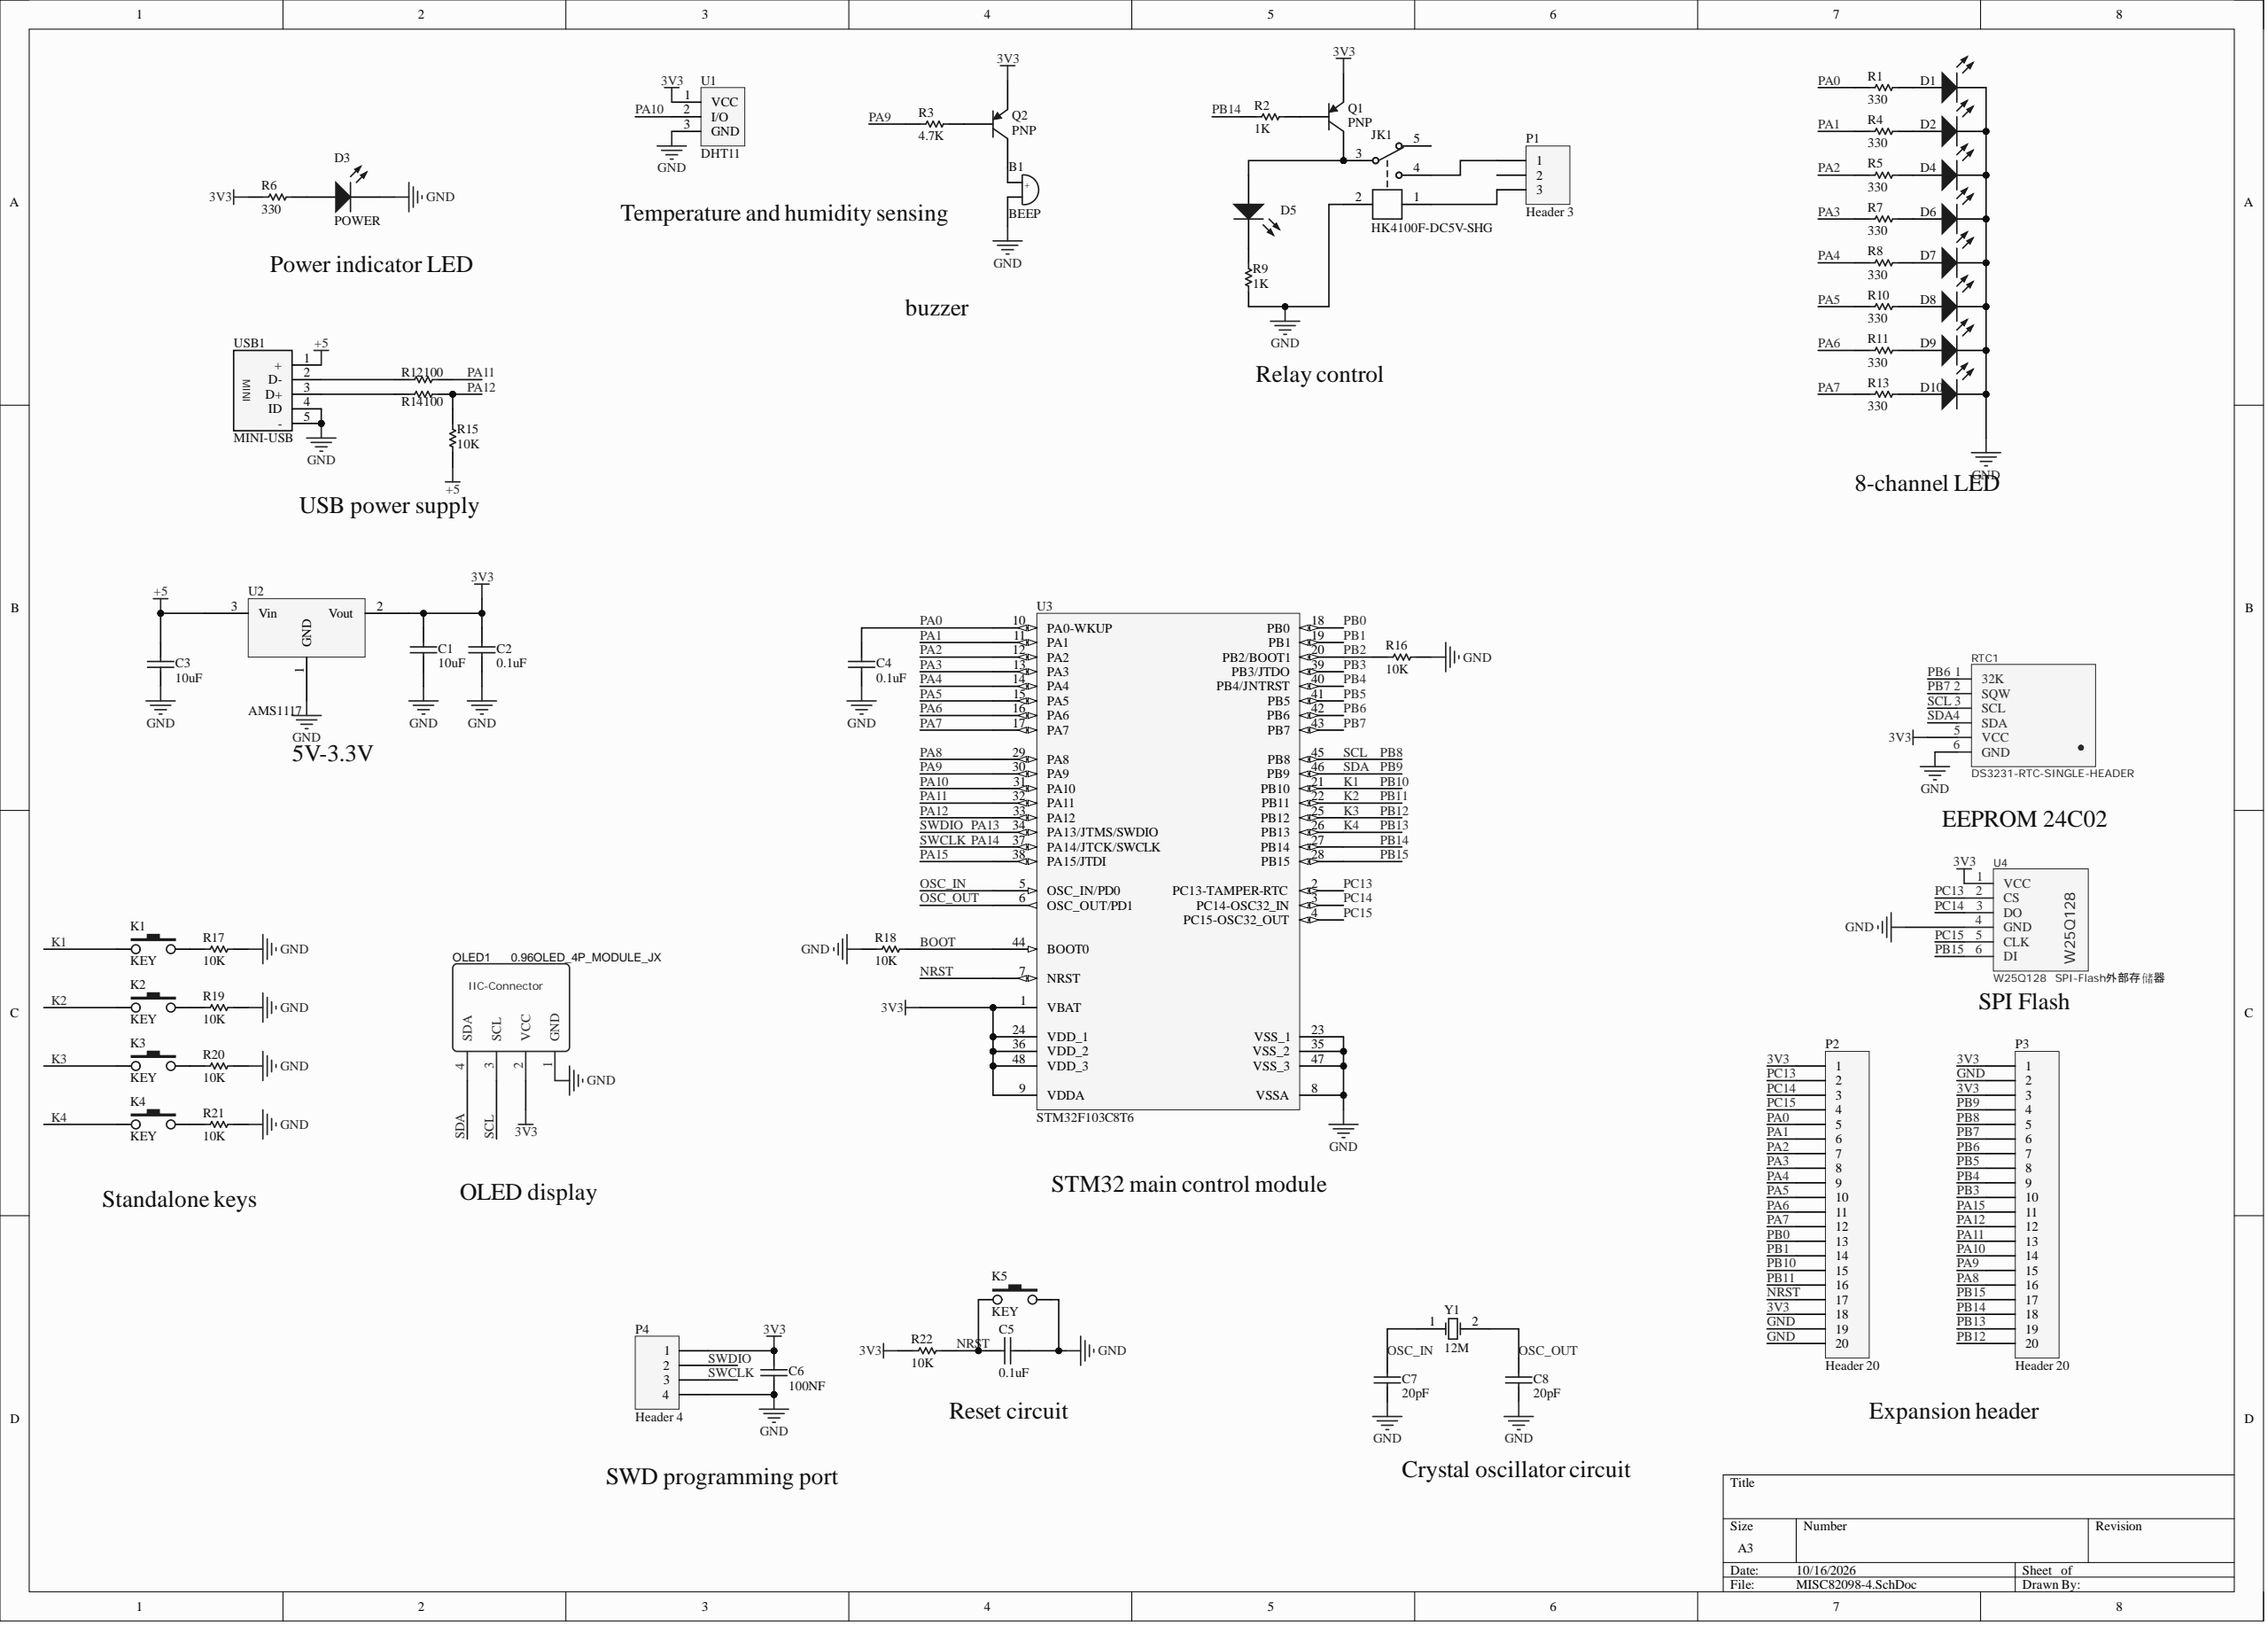Circuit board | Altium Designer | 61 parts | 64 nets
Bill of materials:
Comment,Description,Designator,Footprint,LibRef,Quantity
"BEEP","buzzer","B1","HDR1X2","BEEP","1"
"10uF","non-polarized capacitor","C1, C3","C0603","CAP","2"
"0.1uF","non-polarized capacitor","C2, C4, C5","C0603","CAP","3"
"100NF","non-polarized capacitor","C6","C0603","CAP","1"
"20pF","non-polarized capacitor","C7, C8","C0603","CAP","2"
"POWER","Typical RED, GREEN, YELLOW, AMBER GaAs LED","D1, D2, D3, D4, D5, D6, D7, D8, D9, D10","3.2X1.6X1.1","LED2","10"
"HK4100F-DC5V-SHG","changeover switch set","JK1","HK4100F","HK4100F","1"
"KEY","","K1, K2, K3, K4, K5","DIP-3X6X4.3","KEY","5"
"0.96OLED_4P_MODULE_JX","","OLED1","0.96OLED_4P","0.96OLED_4P_MODULE_JX","1"
"Header 3","Header, 3-Pin","P1","HDR1X3","Header 3","1"
"Header 20","Header, 20-Pin","P2, P3","HDR1X20","Header 20","2"
"Header 4","Header, 4-Pin","P4","HDR1X4","Header 4","1"
"PNP","PNP Bipolar Transistor","Q1, Q2","SOT-23B_N","PNP","2"
"330","","R1, R4, R5, R6, R7, R8, R10, R11, R13","6-0805_N","RES","9"
"1K","","R2, R9","6-0805_N","RES","2"
"4.7K","","R3","6-0805_N","RES","1"
"100","","R12, R14","6-0805_N","RES","2"
"10K","","R15, R16, R17, R18, R19, R20, R21, R22","6-0805_N","RES","8"
"DS3231-RTC-SINGLE-HEADER","","RTC1","DS3231-RTC-24C32-EEPROM-SINGLE-HEADER","DS3231-RTC-SINGLE-HEADER","1"
"DHT11","Header, 3-Pin","U1","HDR1X3","Header 3","1"
"AMS1117","three-terminal voltage regulator","U2","SOT223","AMS1117","1"
"STM32F103C8T6","","U3","LQFP48 7X7","STM32F103C8T6","1"
"W25Q128  SPI-Flash外部存储器","","U4","SPI FLASH","W25Q128  SPI-Flash外部存储器","1"
"MINI-USB","","USB1","USB-MINI-A","MINI-USB","1"
"12M","Crystal Oscillator","Y1","XTAL_US","XTAL","1"
Netlist (Protel format):
[
B1
HDR1X2
BEEP



]
[
C1
C0603
10uF



]
[
C2
C0603
0.1uF



]
[
C3
C0603
10uF



]
[
C4
C0603
0.1uF



]
[
C5
C0603
0.1uF



]
[
C6
C0603
100NF



]
[
C7
C0603
20pF



]
[
C8
C0603
20pF



]
[
D1
3.2X1.6X1.1
POWER



]
[
D2
3.2X1.6X1.1
POWER



]
[
D3
3.2X1.6X1.1
POWER



]
[
D4
3.2X1.6X1.1
POWER



]
[
D5
3.2X1.6X1.1
POWER



]
[
D6
3.2X1.6X1.1
POWER



]
[
D7
3.2X1.6X1.1
POWER



]
[
D8
3.2X1.6X1.1
POWER



]
[
D9
3.2X1.6X1.1
POWER



]
[
D10
3.2X1.6X1.1
POWER



]
[
JK1
HK4100F
HK4100F-DC5V-SHG



]
[
K1
DIP-3X6X4.3
KEY



]
[
K2
DIP-3X6X4.3
KEY



]
[
K3
DIP-3X6X4.3
KEY



]
[
K4
DIP-3X6X4.3
KEY



]
[
K5
DIP-3X6X4.3
KEY



]
[
OLED1
0.96OLED_4P
0.96OLED_4P_MODULE_JX



]
[
P1
HDR1X3
Header 3



]
[
P2
HDR1X20
Header 20



]
[
P3
HDR1X20
Header 20



]
[
P4
HDR1X4
Header 4



]
[
Q1
SOT-23B_N
PNP



]
[
Q2
SOT-23B_N
PNP



]
[
R1
6-0805_N
330



]
[
R2
6-0805_N
1K



]
[
R3
6-0805_N
4.7K



]
[
R4
6-0805_N
330



]
[
R5
6-0805_N
330



]
[
R6
6-0805_N
330



]
[
R7
6-0805_N
330



]
[
R8
6-0805_N
330



]
[
R9
6-0805_N
1K



]
[
R10
6-0805_N
330



]
[
R11
6-0805_N
330



]
[
R12
6-0805_N
100



]
[
R13
6-0805_N
330



]
[
R14
6-0805_N
100



]
[
R15
6-0805_N
10K



]
[
R16
6-0805_N
10K



]
[
R17
6-0805_N
10K



]
[
R18
6-0805_N
10K



]
[
R19
6-0805_N
10K



]
[
R20
6-0805_N
10K



]
[
R21
6-0805_N
10K



]
[
R22
6-0805_N
10K



]
[
RTC1
DS3231-RTC-24C32-EEPROM-SINGLE-HEADER
DS3231-RTC-SINGLE-HEADER



]
[
U1
HDR1X3
DHT11



]
[
U2
SOT223
AMS1117



]
[
U3
LQFP48 7X7
STM32F103C8T6



]
[
U4
SPI FLASH
W25Q128  SPI-Flash外部存储器



]
[
USB1
USB-MINI-A
MINI-USB



]
[
Y1
XTAL_US
12M



]
(
PC15
P2-4
U3-4
U4-5
)
(
PC14
P2-3
U3-3
U4-3
)
(
PC13
P2-2
U3-2
U4-2
)
(
PB15
P3-17
U3-28
U4-6
)
(
PB14
P3-18
R2-2
U3-27
)
(
PB9
OLED1-4
P3-4
RTC1-4
U3-46
)
(
PB8
OLED1-3
P3-5
RTC1-3
U3-45
)
(
PB7
P3-6
RTC1-2
U3-43
)
(
PB6
P3-7
RTC1-1
U3-42
)
(
PB5
P3-8
U3-41
)
(
PB4
P3-9
U3-40
)
(
PB3
P3-10
U3-39
)
(
PB2
R16-2
U3-20
)
(
PB1
P2-14
U3-19
)
(
PB0
P2-13
U3-18
)
(
PA15
P3-11
U3-38
)
(
PA14
P4-3
U3-37
)
(
PA13
P4-2
U3-34
)
(
PA12
P3-12
R14-1
R15-1
U3-33
)
(
PA11
P3-13
R12-1
U3-32
)
(
PA10
P3-14
U1-2
U3-31
)
(
PA9
P3-15
R3-2
U3-30
)
(
PA8
P3-16
U3-29
)
(
PA7
P2-12
R13-2
U3-17
)
(
PA6
P2-11
R11-2
U3-16
)
(
PA5
P2-10
R10-2
U3-15
)
(
PA4
P2-9
R8-2
U3-14
)
(
PA3
P2-8
R7-2
U3-13
)
(
PA2
P2-7
R5-2
U3-12
)
(
PA1
P2-6
R4-2
U3-11
)
(
PA0
C4-2
P2-5
R1-2
U3-10
)
(
OSC_OUT
C8-2
U3-6
Y1-2
)
(
OSC_IN
C7-2
U3-5
Y1-1
)
(
NRST
C5-2
K5-1
P2-17
R22-1
U3-7
)
(
NetR14_2
R14-2
USB1-3
)
(
NetR12_2
R12-2
USB1-2
)
(
NetQ2_2
Q2-2
R3-1
)
(
NetQ1_2
Q1-2
R2-1
)
(
NetK4_3
K4-3
R21-2
)
(
NetK3_3
K3-3
R20-2
)
(
NetK2_3
K2-3
R19-2
)
(
NetK1_3
K1-3
R17-2
)
(
NetJK1_4
JK1-4
P1-1
)
(
NetJK1_1
JK1-1
P1-3
)
(
NetD10_1
D10-1
R13-1
)
(
NetD9_1
D9-1
R11-1
)
(
NetD8_1
D8-1
R10-1
)
(
NetD7_1
D7-1
R8-1
)
(
NetD6_1
D6-1
R7-1
)
(
NetD5_2
D5-2
R9-1
)
(
NetD5_1
D5-1
JK1-3
Q1-1
)
(
NetD4_1
D4-1
R5-1
)
(
NetD3_1
D3-1
R6-1
)
(
NetD2_1
D2-1
R4-1
)
(
NetD1_1
D1-1
R1-1
)
(
NetB1_1
B1-1
Q2-1
)
(
K4
K4-1
P3-19
U3-26
)
(
K3
K3-1
P3-20
U3-25
)
(
K2
K2-1
P2-16
U3-22
)
(
K1
K1-1
P2-15
U3-21
)
(
GND
B1-2
C1-1
C2-1
C3-1
C4-1
C5-1
C6-1
C7-1
C8-1
D1-2
D2-2
D3-2
D4-2
D6-2
D7-2
D8-2
D9-2
D10-2
JK1-2
K5-3
OLED1-1
P2-19
P2-20
P3-2
P4-4
R9-2
R16-1
R17-1
R18-2
R19-1
R20-1
R21-1
RTC1-6
U1-3
U2-1
U3-8
U3-23
U3-35
U3-47
U4-4
USB1-4
USB1-5
)
(
BOOT
R18-1
U3-44
)
(
+5
C3-2
R15-2
U2-3
USB1-1
)
(
3V3
C1-2
C2-2
C6-2
OLED1-2
P2-1
P2-18
P3-1
P3-3
P4-1
Q1-3
Q2-3
R6-2
R22-2
RTC1-5
U1-1
U2-2
U3-1
U3-9
U3-24
U3-36
U3-48
U4-1
)